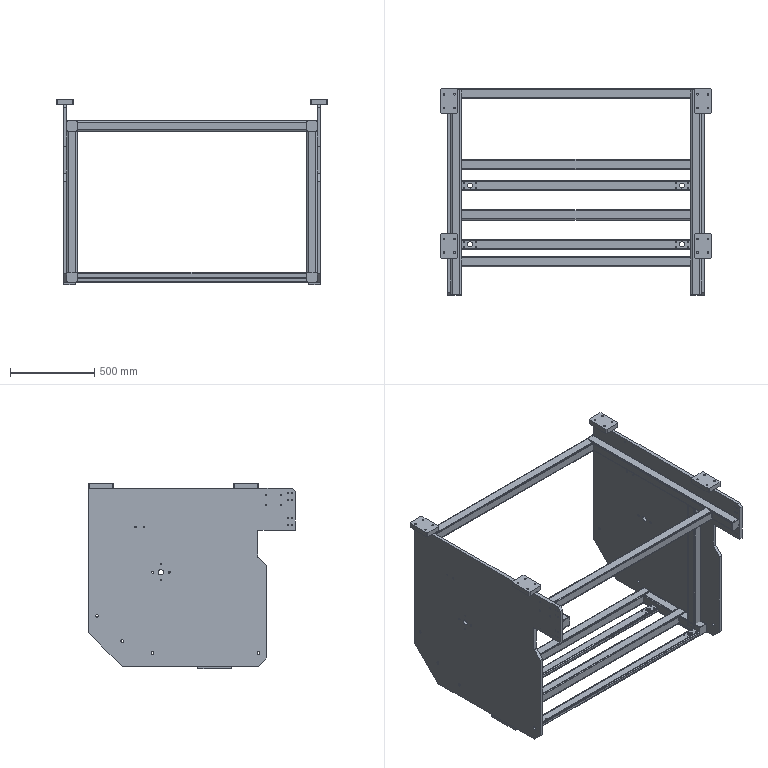Part | SolidWorks | features Chamfer 12, HoleWzd 12, ICE 6, WeldCornerFeat 4, LPattern 3, WeldMemberFeat 3, MirrorPattern 2, EndCap 1, WeldmentFeature 1 | 28 solids | 672 faces | box 1607 x 1230 x 1105 mm | volume 56719734 mm3 | cylinder 384 | plane 256 | cone 32 | commonest cylinder face diameters 5 x80 6.8 x52 6.4 x48 12.8 x48 8.5 x32 10.5 x32